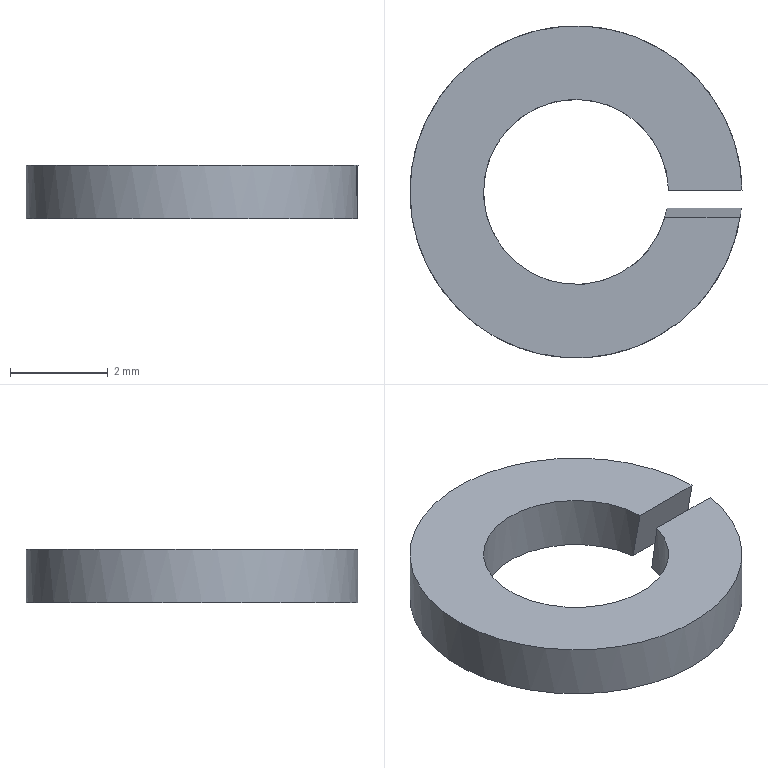Part | NX | features BREP 1 | 1 solid | 6 faces | box 6.78 x 6.78 x 1.1 mm | volume 26.444 mm3 | plane 4 | cylinder 2 | commonest cylinder face diameters 3.78 x1 6.78 x1
STEP:
#1=CARTESIAN_POINT('',(-258.435,-198.172,2104.1));
#2=VERTEX_POINT('',#1);
#3=CARTESIAN_POINT('',(-256.928,-198.172,2104.1));
#4=VERTEX_POINT('',#3);
#5=CARTESIAN_POINT('',(-260.311,-198.172,2104.1));
#6=DIRECTION('',(1.,0.,0.));
#7=VECTOR('',#6,1000.);
#8=LINE('',#5,#7);
#9=EDGE_CURVE('',#2,#4,#8,.T.);
#10=ORIENTED_EDGE('',*,*,#9,.F.);
#11=CARTESIAN_POINT('',(-258.449,-198.731,2104.1));
#12=VERTEX_POINT('',#11);
#13=CARTESIAN_POINT('',(-260.311,-198.403,2104.1));
#14=DIRECTION('',(0.,0.,-1.));
#15=DIRECTION('',(1.,0.,0.));
#16=AXIS2_PLACEMENT_3D('',#13,#14,#15);
#17=CIRCLE('',#16,1.89);
#18=EDGE_CURVE('',#12,#2,#17,.T.);
#19=ORIENTED_EDGE('',*,*,#18,.F.);
#20=CARTESIAN_POINT('',(-256.936,-198.731,2104.1));
#21=VERTEX_POINT('',#20);
#22=CARTESIAN_POINT('',(-260.311,-198.731,2104.1));
#23=DIRECTION('',(-1.,0.,0.));
#24=VECTOR('',#23,1000.);
#25=LINE('',#22,#24);
#26=EDGE_CURVE('',#21,#12,#25,.T.);
#27=ORIENTED_EDGE('',*,*,#26,.F.);
#28=CARTESIAN_POINT('',(-260.311,-198.403,2104.1));
#29=DIRECTION('',(0.,0.,1.));
#30=DIRECTION('',(1.,0.,0.));
#31=AXIS2_PLACEMENT_3D('',#28,#29,#30);
#32=CIRCLE('',#31,3.39);
#33=EDGE_CURVE('',#4,#21,#32,.T.);
#34=ORIENTED_EDGE('',*,*,#33,.F.);
#35=EDGE_LOOP('',(#10,#19,#27,#34));
#36=FACE_BOUND('',#35,.T.);
#37=CARTESIAN_POINT('',(-260.311,-198.403,2104.1));
#38=DIRECTION('',(0.,0.,1.));
#39=DIRECTION('',(-1.,0.,0.));
#40=AXIS2_PLACEMENT_3D('',#37,#38,#39);
#41=PLANE('',#40);
#42=ADVANCED_FACE('',(#36),#41,.F.);
#43=CARTESIAN_POINT('',(-256.921,-198.366,2105.2));
#44=VERTEX_POINT('',#43);
#45=CARTESIAN_POINT('',(-256.921,-198.366,2105.2));
#46=CARTESIAN_POINT('',(-256.921,-198.301,2104.833));
#47=CARTESIAN_POINT('',(-256.924,-198.237,2104.466));
#48=CARTESIAN_POINT('',(-256.928,-198.172,2104.1));
#49=(BOUNDED_CURVE()B_SPLINE_CURVE(3,(#45,#46,#47,#48),.UNSPECIFIED.,.F.,.F.)B_SPLINE_CURVE_WITH_KNOTS((4,4),(0.,1.),.PIECEWISE_BEZIER_KNOTS.)CURVE()GEOMETRIC_REPRESENTATION_ITEM()RATIONAL_B_SPLINE_CURVE((1.,0.9997,0.9997,1.))REPRESENTATION_ITEM(''));
#50=EDGE_CURVE('',#44,#4,#49,.T.);
#51=ORIENTED_EDGE('',*,*,#50,.T.);
#52=ORIENTED_EDGE('',*,*,#33,.T.);
#53=CARTESIAN_POINT('',(-256.961,-198.925,2105.2));
#54=VERTEX_POINT('',#53);
#55=CARTESIAN_POINT('',(-256.936,-198.731,2104.1));
#56=CARTESIAN_POINT('',(-256.943,-198.796,2104.468));
#57=CARTESIAN_POINT('',(-256.951,-198.86,2104.835));
#58=CARTESIAN_POINT('',(-256.961,-198.925,2105.2));
#59=(BOUNDED_CURVE()B_SPLINE_CURVE(3,(#55,#56,#57,#58),.UNSPECIFIED.,.F.,.F.)B_SPLINE_CURVE_WITH_KNOTS((4,4),(0.,1.),.PIECEWISE_BEZIER_KNOTS.)CURVE()GEOMETRIC_REPRESENTATION_ITEM()RATIONAL_B_SPLINE_CURVE((1.,0.9997,0.9997,1.))REPRESENTATION_ITEM(''));
#60=EDGE_CURVE('',#21,#54,#59,.T.);
#61=ORIENTED_EDGE('',*,*,#60,.T.);
#62=CARTESIAN_POINT('',(-260.311,-198.403,2105.2));
#63=DIRECTION('',(0.,0.,-1.));
#64=DIRECTION('',(1.,0.,0.));
#65=AXIS2_PLACEMENT_3D('',#62,#63,#64);
#66=CIRCLE('',#65,3.39);
#67=EDGE_CURVE('',#54,#44,#66,.T.);
#68=ORIENTED_EDGE('',*,*,#67,.T.);
#69=EDGE_LOOP('',(#51,#52,#61,#68));
#70=FACE_BOUND('',#69,.T.);
#71=CARTESIAN_POINT('',(-260.311,-198.403,2104.1));
#72=DIRECTION('',(0.,0.,1.));
#73=DIRECTION('',(-1.,0.,0.));
#74=AXIS2_PLACEMENT_3D('',#71,#72,#73);
#75=CYLINDRICAL_SURFACE('',#74,3.39);
#76=ADVANCED_FACE('',(#70),#75,.T.);
#77=CARTESIAN_POINT('',(-258.421,-198.366,2105.2));
#78=VERTEX_POINT('',#77);
#79=CARTESIAN_POINT('',(-256.921,-198.366,2105.2));
#80=DIRECTION('',(-1.,0.,0.));
#81=VECTOR('',#80,1000.);
#82=LINE('',#79,#81);
#83=EDGE_CURVE('',#44,#78,#82,.T.);
#84=ORIENTED_EDGE('',*,*,#83,.T.);
#85=CARTESIAN_POINT('',(-258.421,-198.366,2105.2));
#86=CARTESIAN_POINT('',(-258.422,-198.301,2104.832));
#87=CARTESIAN_POINT('',(-258.427,-198.237,2104.465));
#88=CARTESIAN_POINT('',(-258.435,-198.172,2104.1));
#89=(BOUNDED_CURVE()B_SPLINE_CURVE(3,(#85,#86,#87,#88),.UNSPECIFIED.,.F.,.F.)B_SPLINE_CURVE_WITH_KNOTS((4,4),(0.,1.),.PIECEWISE_BEZIER_KNOTS.)CURVE()GEOMETRIC_REPRESENTATION_ITEM()RATIONAL_B_SPLINE_CURVE((1.,0.9991,0.9991,1.))REPRESENTATION_ITEM(''));
#90=EDGE_CURVE('',#78,#2,#89,.T.);
#91=ORIENTED_EDGE('',*,*,#90,.T.);
#92=ORIENTED_EDGE('',*,*,#9,.T.);
#93=ORIENTED_EDGE('',*,*,#50,.F.);
#94=EDGE_LOOP('',(#84,#91,#92,#93));
#95=FACE_BOUND('',#94,.T.);
#96=CARTESIAN_POINT('',(-256.921,-197.154,2098.325));
#97=DIRECTION('',(0.,-0.9848,-0.1736));
#98=DIRECTION('',(0.,-0.1736,0.9848));
#99=AXIS2_PLACEMENT_3D('',#96,#97,#98);
#100=PLANE('',#99);
#101=ADVANCED_FACE('',(#95),#100,.T.);
#102=CARTESIAN_POINT('',(-258.494,-198.925,2105.2));
#103=VERTEX_POINT('',#102);
#104=CARTESIAN_POINT('',(-260.311,-198.403,2105.2));
#105=DIRECTION('',(0.,0.,-1.));
#106=DIRECTION('',(1.,0.,0.));
#107=AXIS2_PLACEMENT_3D('',#104,#105,#106);
#108=CIRCLE('',#107,1.89);
#109=EDGE_CURVE('',#103,#78,#108,.T.);
#110=ORIENTED_EDGE('',*,*,#109,.F.);
#111=CARTESIAN_POINT('',(-258.449,-198.731,2104.1));
#112=CARTESIAN_POINT('',(-258.461,-198.796,2104.471));
#113=CARTESIAN_POINT('',(-258.476,-198.861,2104.838));
#114=CARTESIAN_POINT('',(-258.494,-198.925,2105.2));
#115=(BOUNDED_CURVE()B_SPLINE_CURVE(3,(#111,#112,#113,#114),.UNSPECIFIED.,.F.,.F.)B_SPLINE_CURVE_WITH_KNOTS((4,4),(0.,1.),.PIECEWISE_BEZIER_KNOTS.)CURVE()GEOMETRIC_REPRESENTATION_ITEM()RATIONAL_B_SPLINE_CURVE((1.,0.9991,0.9991,1.))REPRESENTATION_ITEM(''));
#116=EDGE_CURVE('',#12,#103,#115,.T.);
#117=ORIENTED_EDGE('',*,*,#116,.F.);
#118=ORIENTED_EDGE('',*,*,#18,.T.);
#119=ORIENTED_EDGE('',*,*,#90,.F.);
#120=EDGE_LOOP('',(#110,#117,#118,#119));
#121=FACE_BOUND('',#120,.T.);
#122=CARTESIAN_POINT('',(-260.311,-198.403,2104.1));
#123=DIRECTION('',(0.,0.,1.));
#124=DIRECTION('',(-1.,0.,0.));
#125=AXIS2_PLACEMENT_3D('',#122,#123,#124);
#126=CYLINDRICAL_SURFACE('',#125,1.89);
#127=ADVANCED_FACE('',(#121),#126,.F.);
#128=ORIENTED_EDGE('',*,*,#26,.T.);
#129=ORIENTED_EDGE('',*,*,#116,.T.);
#130=CARTESIAN_POINT('',(-256.921,-198.925,2105.2));
#131=DIRECTION('',(1.,0.,0.));
#132=VECTOR('',#131,1000.);
#133=LINE('',#130,#132);
#134=EDGE_CURVE('',#103,#54,#133,.T.);
#135=ORIENTED_EDGE('',*,*,#134,.T.);
#136=ORIENTED_EDGE('',*,*,#60,.F.);
#137=EDGE_LOOP('',(#128,#129,#135,#136));
#138=FACE_BOUND('',#137,.T.);
#139=CARTESIAN_POINT('',(-256.921,-197.696,2098.229));
#140=DIRECTION('',(0.,0.9848,0.1736));
#141=DIRECTION('',(0.,0.1736,-0.9848));
#142=AXIS2_PLACEMENT_3D('',#139,#140,#141);
#143=PLANE('',#142);
#144=ADVANCED_FACE('',(#138),#143,.T.);
#145=ORIENTED_EDGE('',*,*,#67,.F.);
#146=ORIENTED_EDGE('',*,*,#134,.F.);
#147=ORIENTED_EDGE('',*,*,#109,.T.);
#148=ORIENTED_EDGE('',*,*,#83,.F.);
#149=EDGE_LOOP('',(#145,#146,#147,#148));
#150=FACE_BOUND('',#149,.T.);
#151=CARTESIAN_POINT('',(-260.311,-198.403,2105.2));
#152=DIRECTION('',(0.,0.,1.));
#153=DIRECTION('',(-1.,0.,0.));
#154=AXIS2_PLACEMENT_3D('',#151,#152,#153);
#155=PLANE('',#154);
#156=ADVANCED_FACE('',(#150),#155,.T.);
#157=CLOSED_SHELL('',(#42,#76,#101,#127,#144,#156));
#158=MANIFOLD_SOLID_BREP('',#157);
#159=(LENGTH_UNIT()NAMED_UNIT(*)SI_UNIT(.MILLI.,.METRE.));
#160=UNCERTAINTY_MEASURE_WITH_UNIT(LENGTH_MEASURE(0.00001),#159,'','');
#161=(NAMED_UNIT(*)PLANE_ANGLE_UNIT()SI_UNIT($,.RADIAN.));
#162=(NAMED_UNIT(*)SI_UNIT($,.STERADIAN.)SOLID_ANGLE_UNIT());
#163=(GEOMETRIC_REPRESENTATION_CONTEXT(3)GLOBAL_UNCERTAINTY_ASSIGNED_CONTEXT((#160))GLOBAL_UNIT_ASSIGNED_CONTEXT((#159,#161,#162))REPRESENTATION_CONTEXT('',''));
#164=ADVANCED_BREP_SHAPE_REPRESENTATION('',(#158),#163);